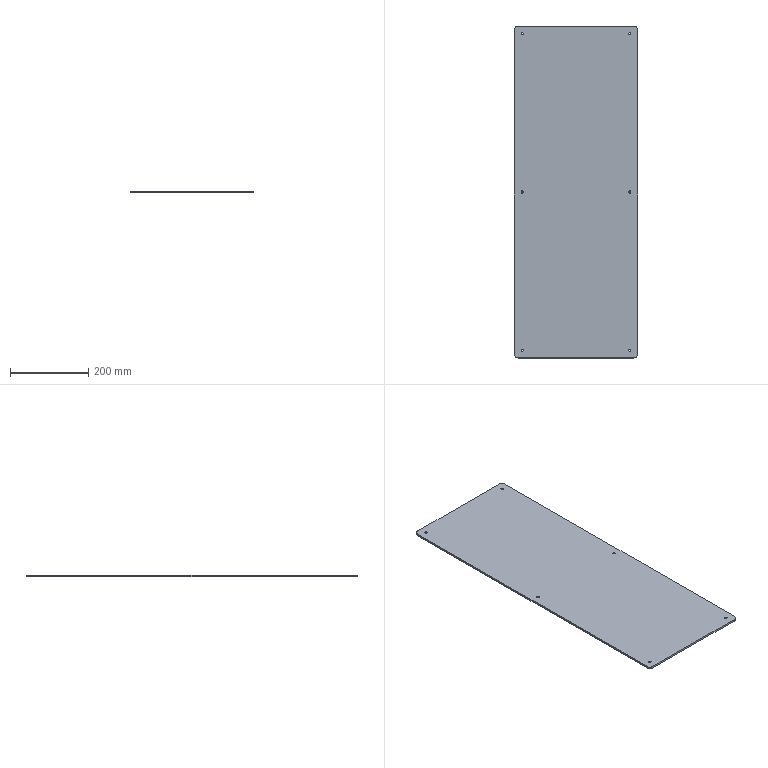Part | SolidWorks | features Extrusion 1, Fillet 1, HoleWzd 1 | 1 solid | 22 faces | box 315 x 850 x 5 mm | volume 1337473 mm3 | cylinder 16 | plane 6 | commonest cylinder face diameters 6 x12 20 x4
STEP:
#1=CARTESIAN_POINT('',(-134.5,405.,0.));
#2=VERTEX_POINT('',#1);
#3=CARTESIAN_POINT('',(-140.5,405.,0.));
#4=VERTEX_POINT('',#3);
#5=CARTESIAN_POINT('',(-137.5,405.,0.));
#6=DIRECTION('',(0.,0.,-1.));
#7=DIRECTION('',(-1.,0.,0.));
#8=AXIS2_PLACEMENT_3D('',#5,#6,#7);
#9=CIRCLE('',#8,3.);
#10=EDGE_CURVE('',#2,#4,#9,.T.);
#11=ORIENTED_EDGE('',*,*,#10,.T.);
#12=CARTESIAN_POINT('',(-140.5,405.,5.));
#13=VERTEX_POINT('',#12);
#14=CARTESIAN_POINT('',(-140.5,405.,5.));
#15=DIRECTION('',(0.,0.,1.));
#16=VECTOR('',#15,1000.);
#17=LINE('',#14,#16);
#18=EDGE_CURVE('',#4,#13,#17,.T.);
#19=ORIENTED_EDGE('',*,*,#18,.T.);
#20=CARTESIAN_POINT('',(-134.5,405.,5.));
#21=VERTEX_POINT('',#20);
#22=CARTESIAN_POINT('',(-137.5,405.,5.));
#23=DIRECTION('',(0.,0.,1.));
#24=DIRECTION('',(1.,0.,0.));
#25=AXIS2_PLACEMENT_3D('',#22,#23,#24);
#26=CIRCLE('',#25,3.);
#27=EDGE_CURVE('',#13,#21,#26,.T.);
#28=ORIENTED_EDGE('',*,*,#27,.T.);
#29=CARTESIAN_POINT('',(-134.5,405.,5.));
#30=DIRECTION('',(0.,0.,1.));
#31=VECTOR('',#30,1000.);
#32=LINE('',#29,#31);
#33=EDGE_CURVE('',#2,#21,#32,.T.);
#34=ORIENTED_EDGE('',*,*,#33,.F.);
#35=EDGE_LOOP('',(#11,#19,#28,#34));
#36=FACE_OUTER_BOUND('',#35,.T.);
#37=CARTESIAN_POINT('',(-137.5,405.,5.));
#38=DIRECTION('',(0.,0.,1.));
#39=DIRECTION('',(1.,0.,0.));
#40=AXIS2_PLACEMENT_3D('',#37,#38,#39);
#41=CYLINDRICAL_SURFACE('',#40,3.);
#42=ADVANCED_FACE('',(#36),#41,.F.);
#43=CARTESIAN_POINT('',(140.5,405.,0.));
#44=VERTEX_POINT('',#43);
#45=CARTESIAN_POINT('',(134.5,405.,0.));
#46=VERTEX_POINT('',#45);
#47=CARTESIAN_POINT('',(137.5,405.,0.));
#48=DIRECTION('',(0.,0.,-1.));
#49=DIRECTION('',(-1.,0.,0.));
#50=AXIS2_PLACEMENT_3D('',#47,#48,#49);
#51=CIRCLE('',#50,3.);
#52=EDGE_CURVE('',#44,#46,#51,.T.);
#53=ORIENTED_EDGE('',*,*,#52,.T.);
#54=CARTESIAN_POINT('',(134.5,405.,5.));
#55=VERTEX_POINT('',#54);
#56=CARTESIAN_POINT('',(134.5,405.,5.));
#57=DIRECTION('',(0.,0.,1.));
#58=VECTOR('',#57,1000.);
#59=LINE('',#56,#58);
#60=EDGE_CURVE('',#46,#55,#59,.T.);
#61=ORIENTED_EDGE('',*,*,#60,.T.);
#62=CARTESIAN_POINT('',(140.5,405.,5.));
#63=VERTEX_POINT('',#62);
#64=CARTESIAN_POINT('',(137.5,405.,5.));
#65=DIRECTION('',(0.,0.,1.));
#66=DIRECTION('',(1.,0.,0.));
#67=AXIS2_PLACEMENT_3D('',#64,#65,#66);
#68=CIRCLE('',#67,3.);
#69=EDGE_CURVE('',#55,#63,#68,.T.);
#70=ORIENTED_EDGE('',*,*,#69,.T.);
#71=CARTESIAN_POINT('',(140.5,405.,5.));
#72=DIRECTION('',(0.,0.,1.));
#73=VECTOR('',#72,1000.);
#74=LINE('',#71,#73);
#75=EDGE_CURVE('',#44,#63,#74,.T.);
#76=ORIENTED_EDGE('',*,*,#75,.F.);
#77=EDGE_LOOP('',(#53,#61,#70,#76));
#78=FACE_OUTER_BOUND('',#77,.T.);
#79=CARTESIAN_POINT('',(137.5,405.,5.));
#80=DIRECTION('',(0.,0.,1.));
#81=DIRECTION('',(1.,0.,0.));
#82=AXIS2_PLACEMENT_3D('',#79,#80,#81);
#83=CYLINDRICAL_SURFACE('',#82,3.);
#84=ADVANCED_FACE('',(#78),#83,.F.);
#85=CARTESIAN_POINT('',(140.5,-405.,0.));
#86=VERTEX_POINT('',#85);
#87=CARTESIAN_POINT('',(134.5,-405.,0.));
#88=VERTEX_POINT('',#87);
#89=CARTESIAN_POINT('',(137.5,-405.,0.));
#90=DIRECTION('',(0.,0.,-1.));
#91=DIRECTION('',(-1.,0.,0.));
#92=AXIS2_PLACEMENT_3D('',#89,#90,#91);
#93=CIRCLE('',#92,3.);
#94=EDGE_CURVE('',#86,#88,#93,.T.);
#95=ORIENTED_EDGE('',*,*,#94,.T.);
#96=CARTESIAN_POINT('',(134.5,-405.,5.));
#97=VERTEX_POINT('',#96);
#98=CARTESIAN_POINT('',(134.5,-405.,5.));
#99=DIRECTION('',(0.,0.,1.));
#100=VECTOR('',#99,1000.);
#101=LINE('',#98,#100);
#102=EDGE_CURVE('',#88,#97,#101,.T.);
#103=ORIENTED_EDGE('',*,*,#102,.T.);
#104=CARTESIAN_POINT('',(140.5,-405.,5.));
#105=VERTEX_POINT('',#104);
#106=CARTESIAN_POINT('',(137.5,-405.,5.));
#107=DIRECTION('',(0.,0.,1.));
#108=DIRECTION('',(1.,0.,0.));
#109=AXIS2_PLACEMENT_3D('',#106,#107,#108);
#110=CIRCLE('',#109,3.);
#111=EDGE_CURVE('',#97,#105,#110,.T.);
#112=ORIENTED_EDGE('',*,*,#111,.T.);
#113=CARTESIAN_POINT('',(140.5,-405.,5.));
#114=DIRECTION('',(0.,0.,1.));
#115=VECTOR('',#114,1000.);
#116=LINE('',#113,#115);
#117=EDGE_CURVE('',#86,#105,#116,.T.);
#118=ORIENTED_EDGE('',*,*,#117,.F.);
#119=EDGE_LOOP('',(#95,#103,#112,#118));
#120=FACE_OUTER_BOUND('',#119,.T.);
#121=CARTESIAN_POINT('',(137.5,-405.,5.));
#122=DIRECTION('',(0.,0.,1.));
#123=DIRECTION('',(1.,0.,0.));
#124=AXIS2_PLACEMENT_3D('',#121,#122,#123);
#125=CYLINDRICAL_SURFACE('',#124,3.);
#126=ADVANCED_FACE('',(#120),#125,.F.);
#127=CARTESIAN_POINT('',(-134.5,-405.,0.));
#128=VERTEX_POINT('',#127);
#129=CARTESIAN_POINT('',(-140.5,-405.,0.));
#130=VERTEX_POINT('',#129);
#131=CARTESIAN_POINT('',(-137.5,-405.,0.));
#132=DIRECTION('',(0.,0.,-1.));
#133=DIRECTION('',(-1.,0.,0.));
#134=AXIS2_PLACEMENT_3D('',#131,#132,#133);
#135=CIRCLE('',#134,3.);
#136=EDGE_CURVE('',#128,#130,#135,.T.);
#137=ORIENTED_EDGE('',*,*,#136,.T.);
#138=CARTESIAN_POINT('',(-140.5,-405.,5.));
#139=VERTEX_POINT('',#138);
#140=CARTESIAN_POINT('',(-140.5,-405.,5.));
#141=DIRECTION('',(0.,0.,1.));
#142=VECTOR('',#141,1000.);
#143=LINE('',#140,#142);
#144=EDGE_CURVE('',#130,#139,#143,.T.);
#145=ORIENTED_EDGE('',*,*,#144,.T.);
#146=CARTESIAN_POINT('',(-134.5,-405.,5.));
#147=VERTEX_POINT('',#146);
#148=CARTESIAN_POINT('',(-137.5,-405.,5.));
#149=DIRECTION('',(0.,0.,1.));
#150=DIRECTION('',(1.,0.,0.));
#151=AXIS2_PLACEMENT_3D('',#148,#149,#150);
#152=CIRCLE('',#151,3.);
#153=EDGE_CURVE('',#139,#147,#152,.T.);
#154=ORIENTED_EDGE('',*,*,#153,.T.);
#155=CARTESIAN_POINT('',(-134.5,-405.,5.));
#156=DIRECTION('',(0.,0.,1.));
#157=VECTOR('',#156,1000.);
#158=LINE('',#155,#157);
#159=EDGE_CURVE('',#128,#147,#158,.T.);
#160=ORIENTED_EDGE('',*,*,#159,.F.);
#161=EDGE_LOOP('',(#137,#145,#154,#160));
#162=FACE_OUTER_BOUND('',#161,.T.);
#163=CARTESIAN_POINT('',(-137.5,-405.,5.));
#164=DIRECTION('',(0.,0.,1.));
#165=DIRECTION('',(1.,0.,0.));
#166=AXIS2_PLACEMENT_3D('',#163,#164,#165);
#167=CYLINDRICAL_SURFACE('',#166,3.);
#168=ADVANCED_FACE('',(#162),#167,.F.);
#169=CARTESIAN_POINT('',(-134.5,0.,0.));
#170=VERTEX_POINT('',#169);
#171=CARTESIAN_POINT('',(-140.5,0.,0.));
#172=VERTEX_POINT('',#171);
#173=CARTESIAN_POINT('',(-137.5,0.,0.));
#174=DIRECTION('',(0.,0.,-1.));
#175=DIRECTION('',(-1.,0.,0.));
#176=AXIS2_PLACEMENT_3D('',#173,#174,#175);
#177=CIRCLE('',#176,3.);
#178=EDGE_CURVE('',#170,#172,#177,.T.);
#179=ORIENTED_EDGE('',*,*,#178,.T.);
#180=CARTESIAN_POINT('',(-140.5,0.,5.));
#181=VERTEX_POINT('',#180);
#182=CARTESIAN_POINT('',(-140.5,0.,5.));
#183=DIRECTION('',(0.,0.,1.));
#184=VECTOR('',#183,1000.);
#185=LINE('',#182,#184);
#186=EDGE_CURVE('',#172,#181,#185,.T.);
#187=ORIENTED_EDGE('',*,*,#186,.T.);
#188=CARTESIAN_POINT('',(-134.5,0.,5.));
#189=VERTEX_POINT('',#188);
#190=CARTESIAN_POINT('',(-137.5,0.,5.));
#191=DIRECTION('',(0.,0.,1.));
#192=DIRECTION('',(1.,0.,0.));
#193=AXIS2_PLACEMENT_3D('',#190,#191,#192);
#194=CIRCLE('',#193,3.);
#195=EDGE_CURVE('',#181,#189,#194,.T.);
#196=ORIENTED_EDGE('',*,*,#195,.T.);
#197=CARTESIAN_POINT('',(-134.5,0.,5.));
#198=DIRECTION('',(0.,0.,1.));
#199=VECTOR('',#198,1000.);
#200=LINE('',#197,#199);
#201=EDGE_CURVE('',#170,#189,#200,.T.);
#202=ORIENTED_EDGE('',*,*,#201,.F.);
#203=EDGE_LOOP('',(#179,#187,#196,#202));
#204=FACE_OUTER_BOUND('',#203,.T.);
#205=CARTESIAN_POINT('',(-137.5,0.,5.));
#206=DIRECTION('',(0.,0.,1.));
#207=DIRECTION('',(1.,0.,0.));
#208=AXIS2_PLACEMENT_3D('',#205,#206,#207);
#209=CYLINDRICAL_SURFACE('',#208,3.);
#210=ADVANCED_FACE('',(#204),#209,.F.);
#211=CARTESIAN_POINT('',(140.5,0.,0.));
#212=VERTEX_POINT('',#211);
#213=CARTESIAN_POINT('',(134.5,0.,0.));
#214=VERTEX_POINT('',#213);
#215=CARTESIAN_POINT('',(137.5,0.,0.));
#216=DIRECTION('',(0.,0.,-1.));
#217=DIRECTION('',(-1.,0.,0.));
#218=AXIS2_PLACEMENT_3D('',#215,#216,#217);
#219=CIRCLE('',#218,3.);
#220=EDGE_CURVE('',#212,#214,#219,.T.);
#221=ORIENTED_EDGE('',*,*,#220,.T.);
#222=CARTESIAN_POINT('',(134.5,0.,5.));
#223=VERTEX_POINT('',#222);
#224=CARTESIAN_POINT('',(134.5,0.,5.));
#225=DIRECTION('',(0.,0.,1.));
#226=VECTOR('',#225,1000.);
#227=LINE('',#224,#226);
#228=EDGE_CURVE('',#214,#223,#227,.T.);
#229=ORIENTED_EDGE('',*,*,#228,.T.);
#230=CARTESIAN_POINT('',(140.5,0.,5.));
#231=VERTEX_POINT('',#230);
#232=CARTESIAN_POINT('',(137.5,0.,5.));
#233=DIRECTION('',(0.,0.,1.));
#234=DIRECTION('',(1.,0.,0.));
#235=AXIS2_PLACEMENT_3D('',#232,#233,#234);
#236=CIRCLE('',#235,3.);
#237=EDGE_CURVE('',#223,#231,#236,.T.);
#238=ORIENTED_EDGE('',*,*,#237,.T.);
#239=CARTESIAN_POINT('',(140.5,0.,5.));
#240=DIRECTION('',(0.,0.,1.));
#241=VECTOR('',#240,1000.);
#242=LINE('',#239,#241);
#243=EDGE_CURVE('',#212,#231,#242,.T.);
#244=ORIENTED_EDGE('',*,*,#243,.F.);
#245=EDGE_LOOP('',(#221,#229,#238,#244));
#246=FACE_OUTER_BOUND('',#245,.T.);
#247=CARTESIAN_POINT('',(137.5,0.,5.));
#248=DIRECTION('',(0.,0.,1.));
#249=DIRECTION('',(1.,0.,0.));
#250=AXIS2_PLACEMENT_3D('',#247,#248,#249);
#251=CYLINDRICAL_SURFACE('',#250,3.);
#252=ADVANCED_FACE('',(#246),#251,.F.);
#253=CARTESIAN_POINT('',(157.5,-415.,5.));
#254=VERTEX_POINT('',#253);
#255=CARTESIAN_POINT('',(157.5,415.,5.));
#256=VERTEX_POINT('',#255);
#257=CARTESIAN_POINT('',(157.5,-425.,5.));
#258=DIRECTION('',(0.,1.,0.));
#259=VECTOR('',#258,1000.);
#260=LINE('',#257,#259);
#261=EDGE_CURVE('',#254,#256,#260,.T.);
#262=ORIENTED_EDGE('',*,*,#261,.F.);
#263=CARTESIAN_POINT('',(157.5,-415.,0.));
#264=VERTEX_POINT('',#263);
#265=CARTESIAN_POINT('',(157.5,-415.,5.));
#266=DIRECTION('',(0.,0.,-1.));
#267=VECTOR('',#266,1000.);
#268=LINE('',#265,#267);
#269=EDGE_CURVE('',#254,#264,#268,.T.);
#270=ORIENTED_EDGE('',*,*,#269,.T.);
#271=CARTESIAN_POINT('',(157.5,415.,0.));
#272=VERTEX_POINT('',#271);
#273=CARTESIAN_POINT('',(157.5,-425.,0.));
#274=DIRECTION('',(0.,1.,0.));
#275=VECTOR('',#274,1000.);
#276=LINE('',#273,#275);
#277=EDGE_CURVE('',#264,#272,#276,.T.);
#278=ORIENTED_EDGE('',*,*,#277,.T.);
#279=CARTESIAN_POINT('',(157.5,415.,5.));
#280=DIRECTION('',(0.,0.,1.));
#281=VECTOR('',#280,1000.);
#282=LINE('',#279,#281);
#283=EDGE_CURVE('',#272,#256,#282,.T.);
#284=ORIENTED_EDGE('',*,*,#283,.T.);
#285=EDGE_LOOP('',(#262,#270,#278,#284));
#286=FACE_OUTER_BOUND('',#285,.T.);
#287=CARTESIAN_POINT('',(157.5,-425.,5.));
#288=DIRECTION('',(-1.,0.,0.));
#289=DIRECTION('',(0.,0.,1.));
#290=AXIS2_PLACEMENT_3D('',#287,#288,#289);
#291=PLANE('',#290);
#292=ADVANCED_FACE('',(#286),#291,.F.);
#293=CARTESIAN_POINT('',(147.5,425.,5.));
#294=VERTEX_POINT('',#293);
#295=CARTESIAN_POINT('',(-147.5,425.,5.));
#296=VERTEX_POINT('',#295);
#297=CARTESIAN_POINT('',(-157.5,425.,5.));
#298=DIRECTION('',(-1.,0.,0.));
#299=VECTOR('',#298,1000.);
#300=LINE('',#297,#299);
#301=EDGE_CURVE('',#294,#296,#300,.T.);
#302=ORIENTED_EDGE('',*,*,#301,.F.);
#303=CARTESIAN_POINT('',(147.5,425.,0.));
#304=VERTEX_POINT('',#303);
#305=CARTESIAN_POINT('',(147.5,425.,5.));
#306=DIRECTION('',(0.,0.,-1.));
#307=VECTOR('',#306,1000.);
#308=LINE('',#305,#307);
#309=EDGE_CURVE('',#294,#304,#308,.T.);
#310=ORIENTED_EDGE('',*,*,#309,.T.);
#311=CARTESIAN_POINT('',(-147.5,425.,0.));
#312=VERTEX_POINT('',#311);
#313=CARTESIAN_POINT('',(-157.5,425.,0.));
#314=DIRECTION('',(-1.,0.,0.));
#315=VECTOR('',#314,1000.);
#316=LINE('',#313,#315);
#317=EDGE_CURVE('',#304,#312,#316,.T.);
#318=ORIENTED_EDGE('',*,*,#317,.T.);
#319=CARTESIAN_POINT('',(-147.5,425.,5.));
#320=DIRECTION('',(0.,0.,1.));
#321=VECTOR('',#320,1000.);
#322=LINE('',#319,#321);
#323=EDGE_CURVE('',#312,#296,#322,.T.);
#324=ORIENTED_EDGE('',*,*,#323,.T.);
#325=EDGE_LOOP('',(#302,#310,#318,#324));
#326=FACE_OUTER_BOUND('',#325,.T.);
#327=CARTESIAN_POINT('',(-157.5,425.,5.));
#328=DIRECTION('',(0.,-1.,0.));
#329=DIRECTION('',(0.,0.,-1.));
#330=AXIS2_PLACEMENT_3D('',#327,#328,#329);
#331=PLANE('',#330);
#332=ADVANCED_FACE('',(#326),#331,.F.);
#333=CARTESIAN_POINT('',(-157.5,415.,0.));
#334=VERTEX_POINT('',#333);
#335=CARTESIAN_POINT('',(-157.5,-415.,0.));
#336=VERTEX_POINT('',#335);
#337=CARTESIAN_POINT('',(-157.5,-425.,0.));
#338=DIRECTION('',(0.,-1.,0.));
#339=VECTOR('',#338,1000.);
#340=LINE('',#337,#339);
#341=EDGE_CURVE('',#334,#336,#340,.T.);
#342=ORIENTED_EDGE('',*,*,#341,.T.);
#343=CARTESIAN_POINT('',(-157.5,-415.,5.));
#344=VERTEX_POINT('',#343);
#345=CARTESIAN_POINT('',(-157.5,-415.,5.));
#346=DIRECTION('',(0.,0.,1.));
#347=VECTOR('',#346,1000.);
#348=LINE('',#345,#347);
#349=EDGE_CURVE('',#336,#344,#348,.T.);
#350=ORIENTED_EDGE('',*,*,#349,.T.);
#351=CARTESIAN_POINT('',(-157.5,415.,5.));
#352=VERTEX_POINT('',#351);
#353=CARTESIAN_POINT('',(-157.5,-425.,5.));
#354=DIRECTION('',(0.,-1.,0.));
#355=VECTOR('',#354,1000.);
#356=LINE('',#353,#355);
#357=EDGE_CURVE('',#352,#344,#356,.T.);
#358=ORIENTED_EDGE('',*,*,#357,.F.);
#359=CARTESIAN_POINT('',(-157.5,415.,5.));
#360=DIRECTION('',(0.,0.,-1.));
#361=VECTOR('',#360,1000.);
#362=LINE('',#359,#361);
#363=EDGE_CURVE('',#352,#334,#362,.T.);
#364=ORIENTED_EDGE('',*,*,#363,.T.);
#365=EDGE_LOOP('',(#342,#350,#358,#364));
#366=FACE_OUTER_BOUND('',#365,.T.);
#367=CARTESIAN_POINT('',(-157.5,-425.,5.));
#368=DIRECTION('',(1.,0.,0.));
#369=DIRECTION('',(0.,0.,-1.));
#370=AXIS2_PLACEMENT_3D('',#367,#368,#369);
#371=PLANE('',#370);
#372=ADVANCED_FACE('',(#366),#371,.F.);
#373=CARTESIAN_POINT('',(-147.5,-425.,5.));
#374=VERTEX_POINT('',#373);
#375=CARTESIAN_POINT('',(147.5,-425.,5.));
#376=VERTEX_POINT('',#375);
#377=CARTESIAN_POINT('',(-157.5,-425.,5.));
#378=DIRECTION('',(1.,0.,0.));
#379=VECTOR('',#378,1000.);
#380=LINE('',#377,#379);
#381=EDGE_CURVE('',#374,#376,#380,.T.);
#382=ORIENTED_EDGE('',*,*,#381,.F.);
#383=CARTESIAN_POINT('',(-147.5,-425.,0.));
#384=VERTEX_POINT('',#383);
#385=CARTESIAN_POINT('',(-147.5,-425.,5.));
#386=DIRECTION('',(0.,0.,-1.));
#387=VECTOR('',#386,1000.);
#388=LINE('',#385,#387);
#389=EDGE_CURVE('',#374,#384,#388,.T.);
#390=ORIENTED_EDGE('',*,*,#389,.T.);
#391=CARTESIAN_POINT('',(147.5,-425.,0.));
#392=VERTEX_POINT('',#391);
#393=CARTESIAN_POINT('',(-157.5,-425.,0.));
#394=DIRECTION('',(1.,0.,0.));
#395=VECTOR('',#394,1000.);
#396=LINE('',#393,#395);
#397=EDGE_CURVE('',#384,#392,#396,.T.);
#398=ORIENTED_EDGE('',*,*,#397,.T.);
#399=CARTESIAN_POINT('',(147.5,-425.,5.));
#400=DIRECTION('',(0.,0.,1.));
#401=VECTOR('',#400,1000.);
#402=LINE('',#399,#401);
#403=EDGE_CURVE('',#392,#376,#402,.T.);
#404=ORIENTED_EDGE('',*,*,#403,.T.);
#405=EDGE_LOOP('',(#382,#390,#398,#404));
#406=FACE_OUTER_BOUND('',#405,.T.);
#407=CARTESIAN_POINT('',(-157.5,-425.,5.));
#408=DIRECTION('',(0.,1.,0.));
#409=DIRECTION('',(0.,0.,1.));
#410=AXIS2_PLACEMENT_3D('',#407,#408,#409);
#411=PLANE('',#410);
#412=ADVANCED_FACE('',(#406),#411,.F.);
#413=CARTESIAN_POINT('',(-137.5,405.,5.));
#414=DIRECTION('',(0.,0.,1.));
#415=DIRECTION('',(1.,0.,0.));
#416=AXIS2_PLACEMENT_3D('',#413,#414,#415);
#417=CIRCLE('',#416,3.);
#418=EDGE_CURVE('',#21,#13,#417,.T.);
#419=ORIENTED_EDGE('',*,*,#418,.F.);
#420=ORIENTED_EDGE('',*,*,#27,.F.);
#421=EDGE_LOOP('',(#419,#420));
#422=FACE_BOUND('',#421,.T.);
#423=CARTESIAN_POINT('',(137.5,405.,5.));
#424=DIRECTION('',(0.,0.,1.));
#425=DIRECTION('',(1.,0.,0.));
#426=AXIS2_PLACEMENT_3D('',#423,#424,#425);
#427=CIRCLE('',#426,3.);
#428=EDGE_CURVE('',#63,#55,#427,.T.);
#429=ORIENTED_EDGE('',*,*,#428,.F.);
#430=ORIENTED_EDGE('',*,*,#69,.F.);
#431=EDGE_LOOP('',(#429,#430));
#432=FACE_BOUND('',#431,.T.);
#433=CARTESIAN_POINT('',(137.5,-405.,5.));
#434=DIRECTION('',(0.,0.,1.));
#435=DIRECTION('',(1.,0.,0.));
#436=AXIS2_PLACEMENT_3D('',#433,#434,#435);
#437=CIRCLE('',#436,3.);
#438=EDGE_CURVE('',#105,#97,#437,.T.);
#439=ORIENTED_EDGE('',*,*,#438,.F.);
#440=ORIENTED_EDGE('',*,*,#111,.F.);
#441=EDGE_LOOP('',(#439,#440));
#442=FACE_BOUND('',#441,.T.);
#443=CARTESIAN_POINT('',(-137.5,-405.,5.));
#444=DIRECTION('',(0.,0.,1.));
#445=DIRECTION('',(1.,0.,0.));
#446=AXIS2_PLACEMENT_3D('',#443,#444,#445);
#447=CIRCLE('',#446,3.);
#448=EDGE_CURVE('',#147,#139,#447,.T.);
#449=ORIENTED_EDGE('',*,*,#448,.F.);
#450=ORIENTED_EDGE('',*,*,#153,.F.);
#451=EDGE_LOOP('',(#449,#450));
#452=FACE_BOUND('',#451,.T.);
#453=CARTESIAN_POINT('',(-137.5,0.,5.));
#454=DIRECTION('',(0.,0.,1.));
#455=DIRECTION('',(1.,0.,0.));
#456=AXIS2_PLACEMENT_3D('',#453,#454,#455);
#457=CIRCLE('',#456,3.);
#458=EDGE_CURVE('',#189,#181,#457,.T.);
#459=ORIENTED_EDGE('',*,*,#458,.F.);
#460=ORIENTED_EDGE('',*,*,#195,.F.);
#461=EDGE_LOOP('',(#459,#460));
#462=FACE_BOUND('',#461,.T.);
#463=CARTESIAN_POINT('',(137.5,0.,5.));
#464=DIRECTION('',(0.,0.,1.));
#465=DIRECTION('',(1.,0.,0.));
#466=AXIS2_PLACEMENT_3D('',#463,#464,#465);
#467=CIRCLE('',#466,3.);
#468=EDGE_CURVE('',#231,#223,#467,.T.);
#469=ORIENTED_EDGE('',*,*,#468,.F.);
#470=ORIENTED_EDGE('',*,*,#237,.F.);
#471=EDGE_LOOP('',(#469,#470));
#472=FACE_BOUND('',#471,.T.);
#473=ORIENTED_EDGE('',*,*,#357,.T.);
#474=CARTESIAN_POINT('',(-147.5,-415.,5.));
#475=DIRECTION('',(0.,0.,1.));
#476=DIRECTION('',(-1.,0.,0.));
#477=AXIS2_PLACEMENT_3D('',#474,#475,#476);
#478=CIRCLE('',#477,10.);
#479=EDGE_CURVE('',#344,#374,#478,.T.);
#480=ORIENTED_EDGE('',*,*,#479,.T.);
#481=ORIENTED_EDGE('',*,*,#381,.T.);
#482=CARTESIAN_POINT('',(147.5,-415.,5.));
#483=DIRECTION('',(0.,0.,1.));
#484=DIRECTION('',(-1.,0.,0.));
#485=AXIS2_PLACEMENT_3D('',#482,#483,#484);
#486=CIRCLE('',#485,10.);
#487=EDGE_CURVE('',#376,#254,#486,.T.);
#488=ORIENTED_EDGE('',*,*,#487,.T.);
#489=ORIENTED_EDGE('',*,*,#261,.T.);
#490=CARTESIAN_POINT('',(147.5,415.,5.));
#491=DIRECTION('',(0.,0.,1.));
#492=DIRECTION('',(-1.,0.,0.));
#493=AXIS2_PLACEMENT_3D('',#490,#491,#492);
#494=CIRCLE('',#493,10.);
#495=EDGE_CURVE('',#256,#294,#494,.T.);
#496=ORIENTED_EDGE('',*,*,#495,.T.);
#497=ORIENTED_EDGE('',*,*,#301,.T.);
#498=CARTESIAN_POINT('',(-147.5,415.,5.));
#499=DIRECTION('',(0.,0.,1.));
#500=DIRECTION('',(-1.,0.,0.));
#501=AXIS2_PLACEMENT_3D('',#498,#499,#500);
#502=CIRCLE('',#501,10.);
#503=EDGE_CURVE('',#296,#352,#502,.T.);
#504=ORIENTED_EDGE('',*,*,#503,.T.);
#505=EDGE_LOOP('',(#473,#480,#481,#488,#489,#496,#497,#504));
#506=FACE_OUTER_BOUND('',#505,.T.);
#507=CARTESIAN_POINT('',(0.,0.,5.));
#508=DIRECTION('',(0.,0.,-1.));
#509=DIRECTION('',(-1.,0.,0.));
#510=AXIS2_PLACEMENT_3D('',#507,#508,#509);
#511=PLANE('',#510);
#512=ADVANCED_FACE('',(#422,#432,#442,#452,#462,#472,#506),#511,.F.);
#513=ORIENTED_EDGE('',*,*,#10,.F.);
#514=CARTESIAN_POINT('',(-137.5,405.,0.));
#515=DIRECTION('',(0.,0.,-1.));
#516=DIRECTION('',(-1.,0.,0.));
#517=AXIS2_PLACEMENT_3D('',#514,#515,#516);
#518=CIRCLE('',#517,3.);
#519=EDGE_CURVE('',#4,#2,#518,.T.);
#520=ORIENTED_EDGE('',*,*,#519,.F.);
#521=EDGE_LOOP('',(#513,#520));
#522=FACE_BOUND('',#521,.T.);
#523=ORIENTED_EDGE('',*,*,#52,.F.);
#524=CARTESIAN_POINT('',(137.5,405.,0.));
#525=DIRECTION('',(0.,0.,-1.));
#526=DIRECTION('',(-1.,0.,0.));
#527=AXIS2_PLACEMENT_3D('',#524,#525,#526);
#528=CIRCLE('',#527,3.);
#529=EDGE_CURVE('',#46,#44,#528,.T.);
#530=ORIENTED_EDGE('',*,*,#529,.F.);
#531=EDGE_LOOP('',(#523,#530));
#532=FACE_BOUND('',#531,.T.);
#533=ORIENTED_EDGE('',*,*,#94,.F.);
#534=CARTESIAN_POINT('',(137.5,-405.,0.));
#535=DIRECTION('',(0.,0.,-1.));
#536=DIRECTION('',(-1.,0.,0.));
#537=AXIS2_PLACEMENT_3D('',#534,#535,#536);
#538=CIRCLE('',#537,3.);
#539=EDGE_CURVE('',#88,#86,#538,.T.);
#540=ORIENTED_EDGE('',*,*,#539,.F.);
#541=EDGE_LOOP('',(#533,#540));
#542=FACE_BOUND('',#541,.T.);
#543=ORIENTED_EDGE('',*,*,#136,.F.);
#544=CARTESIAN_POINT('',(-137.5,-405.,0.));
#545=DIRECTION('',(0.,0.,-1.));
#546=DIRECTION('',(-1.,0.,0.));
#547=AXIS2_PLACEMENT_3D('',#544,#545,#546);
#548=CIRCLE('',#547,3.);
#549=EDGE_CURVE('',#130,#128,#548,.T.);
#550=ORIENTED_EDGE('',*,*,#549,.F.);
#551=EDGE_LOOP('',(#543,#550));
#552=FACE_BOUND('',#551,.T.);
#553=ORIENTED_EDGE('',*,*,#178,.F.);
#554=CARTESIAN_POINT('',(-137.5,0.,0.));
#555=DIRECTION('',(0.,0.,-1.));
#556=DIRECTION('',(-1.,0.,0.));
#557=AXIS2_PLACEMENT_3D('',#554,#555,#556);
#558=CIRCLE('',#557,3.);
#559=EDGE_CURVE('',#172,#170,#558,.T.);
#560=ORIENTED_EDGE('',*,*,#559,.F.);
#561=EDGE_LOOP('',(#553,#560));
#562=FACE_BOUND('',#561,.T.);
#563=ORIENTED_EDGE('',*,*,#220,.F.);
#564=CARTESIAN_POINT('',(137.5,0.,0.));
#565=DIRECTION('',(0.,0.,-1.));
#566=DIRECTION('',(-1.,0.,0.));
#567=AXIS2_PLACEMENT_3D('',#564,#565,#566);
#568=CIRCLE('',#567,3.);
#569=EDGE_CURVE('',#214,#212,#568,.T.);
#570=ORIENTED_EDGE('',*,*,#569,.F.);
#571=EDGE_LOOP('',(#563,#570));
#572=FACE_BOUND('',#571,.T.);
#573=ORIENTED_EDGE('',*,*,#397,.F.);
#574=CARTESIAN_POINT('',(-147.5,-415.,0.));
#575=DIRECTION('',(0.,0.,-1.));
#576=DIRECTION('',(-1.,0.,0.));
#577=AXIS2_PLACEMENT_3D('',#574,#575,#576);
#578=CIRCLE('',#577,10.);
#579=EDGE_CURVE('',#384,#336,#578,.T.);
#580=ORIENTED_EDGE('',*,*,#579,.T.);
#581=ORIENTED_EDGE('',*,*,#341,.F.);
#582=CARTESIAN_POINT('',(-147.5,415.,0.));
#583=DIRECTION('',(0.,0.,-1.));
#584=DIRECTION('',(-1.,0.,0.));
#585=AXIS2_PLACEMENT_3D('',#582,#583,#584);
#586=CIRCLE('',#585,10.);
#587=EDGE_CURVE('',#334,#312,#586,.T.);
#588=ORIENTED_EDGE('',*,*,#587,.T.);
#589=ORIENTED_EDGE('',*,*,#317,.F.);
#590=CARTESIAN_POINT('',(147.5,415.,0.));
#591=DIRECTION('',(0.,0.,-1.));
#592=DIRECTION('',(-1.,0.,0.));
#593=AXIS2_PLACEMENT_3D('',#590,#591,#592);
#594=CIRCLE('',#593,10.);
#595=EDGE_CURVE('',#304,#272,#594,.T.);
#596=ORIENTED_EDGE('',*,*,#595,.T.);
#597=ORIENTED_EDGE('',*,*,#277,.F.);
#598=CARTESIAN_POINT('',(147.5,-415.,0.));
#599=DIRECTION('',(0.,0.,-1.));
#600=DIRECTION('',(-1.,0.,0.));
#601=AXIS2_PLACEMENT_3D('',#598,#599,#600);
#602=CIRCLE('',#601,10.);
#603=EDGE_CURVE('',#264,#392,#602,.T.);
#604=ORIENTED_EDGE('',*,*,#603,.T.);
#605=EDGE_LOOP('',(#573,#580,#581,#588,#589,#596,#597,#604));
#606=FACE_OUTER_BOUND('',#605,.T.);
#607=CARTESIAN_POINT('',(0.,0.,0.));
#608=DIRECTION('',(0.,0.,-1.));
#609=DIRECTION('',(-1.,0.,0.));
#610=AXIS2_PLACEMENT_3D('',#607,#608,#609);
#611=PLANE('',#610);
#612=ADVANCED_FACE('',(#522,#532,#542,#552,#562,#572,#606),#611,.T.);
#613=ORIENTED_EDGE('',*,*,#228,.F.);
#614=ORIENTED_EDGE('',*,*,#569,.T.);
#615=ORIENTED_EDGE('',*,*,#243,.T.);
#616=ORIENTED_EDGE('',*,*,#468,.T.);
#617=EDGE_LOOP('',(#613,#614,#615,#616));
#618=FACE_OUTER_BOUND('',#617,.T.);
#619=CARTESIAN_POINT('',(137.5,0.,5.));
#620=DIRECTION('',(0.,0.,1.));
#621=DIRECTION('',(1.,0.,0.));
#622=AXIS2_PLACEMENT_3D('',#619,#620,#621);
#623=CYLINDRICAL_SURFACE('',#622,3.);
#624=ADVANCED_FACE('',(#618),#623,.F.);
#625=ORIENTED_EDGE('',*,*,#186,.F.);
#626=ORIENTED_EDGE('',*,*,#559,.T.);
#627=ORIENTED_EDGE('',*,*,#201,.T.);
#628=ORIENTED_EDGE('',*,*,#458,.T.);
#629=EDGE_LOOP('',(#625,#626,#627,#628));
#630=FACE_OUTER_BOUND('',#629,.T.);
#631=CARTESIAN_POINT('',(-137.5,0.,5.));
#632=DIRECTION('',(0.,0.,1.));
#633=DIRECTION('',(1.,0.,0.));
#634=AXIS2_PLACEMENT_3D('',#631,#632,#633);
#635=CYLINDRICAL_SURFACE('',#634,3.);
#636=ADVANCED_FACE('',(#630),#635,.F.);
#637=ORIENTED_EDGE('',*,*,#144,.F.);
#638=ORIENTED_EDGE('',*,*,#549,.T.);
#639=ORIENTED_EDGE('',*,*,#159,.T.);
#640=ORIENTED_EDGE('',*,*,#448,.T.);
#641=EDGE_LOOP('',(#637,#638,#639,#640));
#642=FACE_OUTER_BOUND('',#641,.T.);
#643=CARTESIAN_POINT('',(-137.5,-405.,5.));
#644=DIRECTION('',(0.,0.,1.));
#645=DIRECTION('',(1.,0.,0.));
#646=AXIS2_PLACEMENT_3D('',#643,#644,#645);
#647=CYLINDRICAL_SURFACE('',#646,3.);
#648=ADVANCED_FACE('',(#642),#647,.F.);
#649=ORIENTED_EDGE('',*,*,#102,.F.);
#650=ORIENTED_EDGE('',*,*,#539,.T.);
#651=ORIENTED_EDGE('',*,*,#117,.T.);
#652=ORIENTED_EDGE('',*,*,#438,.T.);
#653=EDGE_LOOP('',(#649,#650,#651,#652));
#654=FACE_OUTER_BOUND('',#653,.T.);
#655=CARTESIAN_POINT('',(137.5,-405.,5.));
#656=DIRECTION('',(0.,0.,1.));
#657=DIRECTION('',(1.,0.,0.));
#658=AXIS2_PLACEMENT_3D('',#655,#656,#657);
#659=CYLINDRICAL_SURFACE('',#658,3.);
#660=ADVANCED_FACE('',(#654),#659,.F.);
#661=ORIENTED_EDGE('',*,*,#60,.F.);
#662=ORIENTED_EDGE('',*,*,#529,.T.);
#663=ORIENTED_EDGE('',*,*,#75,.T.);
#664=ORIENTED_EDGE('',*,*,#428,.T.);
#665=EDGE_LOOP('',(#661,#662,#663,#664));
#666=FACE_OUTER_BOUND('',#665,.T.);
#667=CARTESIAN_POINT('',(137.5,405.,5.));
#668=DIRECTION('',(0.,0.,1.));
#669=DIRECTION('',(1.,0.,0.));
#670=AXIS2_PLACEMENT_3D('',#667,#668,#669);
#671=CYLINDRICAL_SURFACE('',#670,3.);
#672=ADVANCED_FACE('',(#666),#671,.F.);
#673=ORIENTED_EDGE('',*,*,#18,.F.);
#674=ORIENTED_EDGE('',*,*,#519,.T.);
#675=ORIENTED_EDGE('',*,*,#33,.T.);
#676=ORIENTED_EDGE('',*,*,#418,.T.);
#677=EDGE_LOOP('',(#673,#674,#675,#676));
#678=FACE_OUTER_BOUND('',#677,.T.);
#679=CARTESIAN_POINT('',(-137.5,405.,5.));
#680=DIRECTION('',(0.,0.,1.));
#681=DIRECTION('',(1.,0.,0.));
#682=AXIS2_PLACEMENT_3D('',#679,#680,#681);
#683=CYLINDRICAL_SURFACE('',#682,3.);
#684=ADVANCED_FACE('',(#678),#683,.F.);
#685=ORIENTED_EDGE('',*,*,#479,.F.);
#686=ORIENTED_EDGE('',*,*,#349,.F.);
#687=ORIENTED_EDGE('',*,*,#579,.F.);
#688=ORIENTED_EDGE('',*,*,#389,.F.);
#689=EDGE_LOOP('',(#685,#686,#687,#688));
#690=FACE_OUTER_BOUND('',#689,.T.);
#691=CARTESIAN_POINT('',(-147.5,-415.,5.));
#692=DIRECTION('',(0.,0.,-1.));
#693=DIRECTION('',(-1.,0.,0.));
#694=AXIS2_PLACEMENT_3D('',#691,#692,#693);
#695=CYLINDRICAL_SURFACE('',#694,10.);
#696=ADVANCED_FACE('',(#690),#695,.T.);
#697=ORIENTED_EDGE('',*,*,#487,.F.);
#698=ORIENTED_EDGE('',*,*,#403,.F.);
#699=ORIENTED_EDGE('',*,*,#603,.F.);
#700=ORIENTED_EDGE('',*,*,#269,.F.);
#701=EDGE_LOOP('',(#697,#698,#699,#700));
#702=FACE_OUTER_BOUND('',#701,.T.);
#703=CARTESIAN_POINT('',(147.5,-415.,5.));
#704=DIRECTION('',(0.,0.,-1.));
#705=DIRECTION('',(-1.,0.,0.));
#706=AXIS2_PLACEMENT_3D('',#703,#704,#705);
#707=CYLINDRICAL_SURFACE('',#706,10.);
#708=ADVANCED_FACE('',(#702),#707,.T.);
#709=ORIENTED_EDGE('',*,*,#495,.F.);
#710=ORIENTED_EDGE('',*,*,#283,.F.);
#711=ORIENTED_EDGE('',*,*,#595,.F.);
#712=ORIENTED_EDGE('',*,*,#309,.F.);
#713=EDGE_LOOP('',(#709,#710,#711,#712));
#714=FACE_OUTER_BOUND('',#713,.T.);
#715=CARTESIAN_POINT('',(147.5,415.,5.));
#716=DIRECTION('',(0.,0.,-1.));
#717=DIRECTION('',(-1.,0.,0.));
#718=AXIS2_PLACEMENT_3D('',#715,#716,#717);
#719=CYLINDRICAL_SURFACE('',#718,10.);
#720=ADVANCED_FACE('',(#714),#719,.T.);
#721=ORIENTED_EDGE('',*,*,#503,.F.);
#722=ORIENTED_EDGE('',*,*,#323,.F.);
#723=ORIENTED_EDGE('',*,*,#587,.F.);
#724=ORIENTED_EDGE('',*,*,#363,.F.);
#725=EDGE_LOOP('',(#721,#722,#723,#724));
#726=FACE_OUTER_BOUND('',#725,.T.);
#727=CARTESIAN_POINT('',(-147.5,415.,5.));
#728=DIRECTION('',(0.,0.,-1.));
#729=DIRECTION('',(-1.,0.,0.));
#730=AXIS2_PLACEMENT_3D('',#727,#728,#729);
#731=CYLINDRICAL_SURFACE('',#730,10.);
#732=ADVANCED_FACE('',(#726),#731,.T.);
#733=CLOSED_SHELL('',(#42,#84,#126,#168,#210,#252,#292,#332,#372,#412,#512,#612,#624,#636,#648,#660,#672,#684,#696,#708,#720,#732));
#734=MANIFOLD_SOLID_BREP('',#733);
#735=CARTESIAN_POINT('',(0.,0.,0.));
#736=DIRECTION('',(0.,0.,1.));
#737=DIRECTION('',(1.,0.,0.));
#738=AXIS2_PLACEMENT_3D('',#735,#736,#737);
#739=(LENGTH_UNIT()NAMED_UNIT(*)SI_UNIT(.MILLI.,.METRE.));
#740=UNCERTAINTY_MEASURE_WITH_UNIT(LENGTH_MEASURE(0.00001),#739,'','');
#741=(NAMED_UNIT(*)PLANE_ANGLE_UNIT()SI_UNIT($,.RADIAN.));
#742=(NAMED_UNIT(*)SI_UNIT($,.STERADIAN.)SOLID_ANGLE_UNIT());
#743=(GEOMETRIC_REPRESENTATION_CONTEXT(3)GLOBAL_UNCERTAINTY_ASSIGNED_CONTEXT((#740))GLOBAL_UNIT_ASSIGNED_CONTEXT((#739,#741,#742))REPRESENTATION_CONTEXT('',''));
#744=ADVANCED_BREP_SHAPE_REPRESENTATION('',(#734,#738),#743);